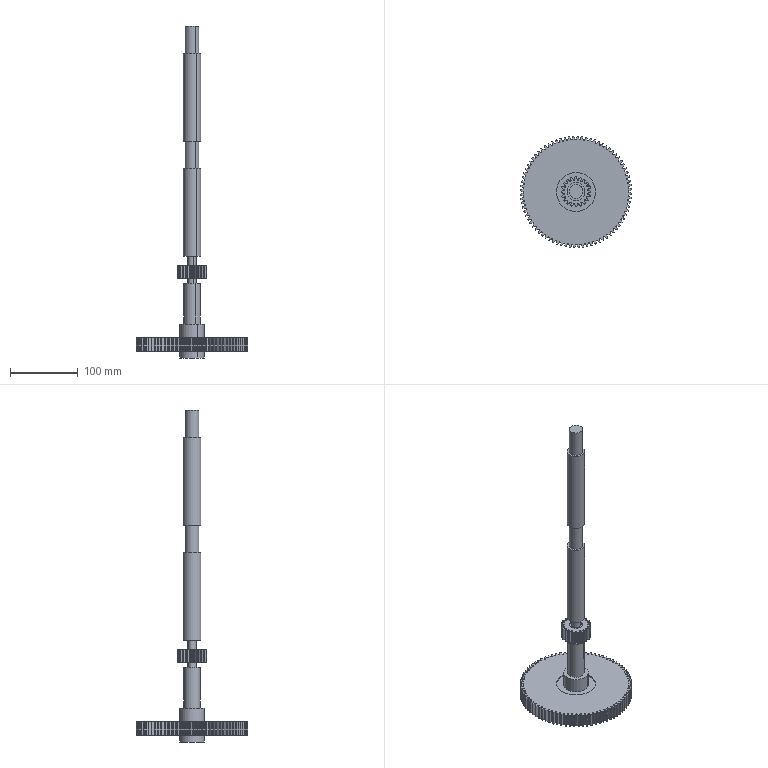Part | SolidWorks | features RefAxis 2 | 5 solids | 773 faces | box 163.961 x 163.961 x 490 mm | volume 641147 mm3 | cylinder 491 | spline 200 | plane 82 | commonest cylinder face diameters 1.52 x244 155 x81 164 x80 35 x21 44 x20 5 x6